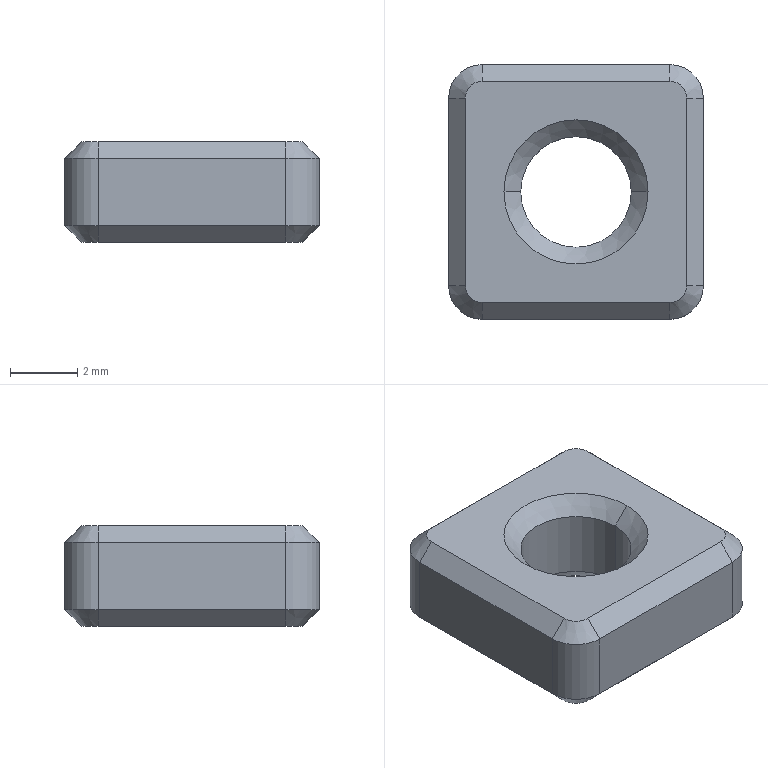Part | SolidWorks | features Chamfer 3, Extrusion 1, HoleWzd 1 | 1 solid | 32 faces | box 7.6 x 7.6 x 3 mm | volume 135.283 mm3 | plane 14 | cone 12 | cylinder 6 | commonest cylinder face diameters 2 x4 3.3 x2
STEP:
#1=CARTESIAN_POINT('',(-1.65,0.,2.5));
#2=VERTEX_POINT('',#1);
#3=CARTESIAN_POINT('',(1.65,0.,2.5));
#4=VERTEX_POINT('',#3);
#5=CARTESIAN_POINT('',(0.,0.,2.5));
#6=DIRECTION('',(0.,0.,1.));
#7=DIRECTION('',(1.,0.,0.));
#8=AXIS2_PLACEMENT_3D('',#5,#6,#7);
#9=CIRCLE('',#8,1.65);
#10=EDGE_CURVE('',#2,#4,#9,.T.);
#11=ORIENTED_EDGE('',*,*,#10,.F.);
#12=CARTESIAN_POINT('',(-2.15,0.,3.));
#13=VERTEX_POINT('',#12);
#14=CARTESIAN_POINT('',(-1.65,0.,2.5));
#15=DIRECTION('',(-0.7071,0.,0.7071));
#16=VECTOR('',#15,1000.);
#17=LINE('',#14,#16);
#18=EDGE_CURVE('',#2,#13,#17,.T.);
#19=ORIENTED_EDGE('',*,*,#18,.T.);
#20=CARTESIAN_POINT('',(2.15,0.,3.));
#21=VERTEX_POINT('',#20);
#22=CARTESIAN_POINT('',(0.,0.,3.));
#23=DIRECTION('',(0.,0.,-1.));
#24=DIRECTION('',(1.,0.,0.));
#25=AXIS2_PLACEMENT_3D('',#22,#23,#24);
#26=CIRCLE('',#25,2.15);
#27=EDGE_CURVE('',#21,#13,#26,.T.);
#28=ORIENTED_EDGE('',*,*,#27,.F.);
#29=CARTESIAN_POINT('',(1.65,0.,2.5));
#30=DIRECTION('',(0.7071,0.,0.7071));
#31=VECTOR('',#30,1000.);
#32=LINE('',#29,#31);
#33=EDGE_CURVE('',#4,#21,#32,.T.);
#34=ORIENTED_EDGE('',*,*,#33,.F.);
#35=EDGE_LOOP('',(#11,#19,#28,#34));
#36=FACE_OUTER_BOUND('',#35,.T.);
#37=CARTESIAN_POINT('',(0.,0.,2.5));
#38=DIRECTION('',(0.,0.,1.));
#39=DIRECTION('',(1.,0.,0.));
#40=AXIS2_PLACEMENT_3D('',#37,#38,#39);
#41=CONICAL_SURFACE('',#40,1.65,0.7854);
#42=ADVANCED_FACE('',(#36),#41,.F.);
#43=CARTESIAN_POINT('',(1.65,0.,0.5));
#44=VERTEX_POINT('',#43);
#45=CARTESIAN_POINT('',(-1.65,0.,0.5));
#46=VERTEX_POINT('',#45);
#47=CARTESIAN_POINT('',(0.,0.,0.5));
#48=DIRECTION('',(0.,0.,-1.));
#49=DIRECTION('',(1.,0.,0.));
#50=AXIS2_PLACEMENT_3D('',#47,#48,#49);
#51=CIRCLE('',#50,1.65);
#52=EDGE_CURVE('',#44,#46,#51,.T.);
#53=ORIENTED_EDGE('',*,*,#52,.F.);
#54=CARTESIAN_POINT('',(2.15,0.,0.));
#55=VERTEX_POINT('',#54);
#56=CARTESIAN_POINT('',(1.65,0.,0.5));
#57=DIRECTION('',(0.7071,0.,-0.7071));
#58=VECTOR('',#57,1000.);
#59=LINE('',#56,#58);
#60=EDGE_CURVE('',#44,#55,#59,.T.);
#61=ORIENTED_EDGE('',*,*,#60,.T.);
#62=CARTESIAN_POINT('',(-2.15,0.,0.));
#63=VERTEX_POINT('',#62);
#64=CARTESIAN_POINT('',(0.,0.,0.));
#65=DIRECTION('',(0.,0.,1.));
#66=DIRECTION('',(1.,0.,0.));
#67=AXIS2_PLACEMENT_3D('',#64,#65,#66);
#68=CIRCLE('',#67,2.15);
#69=EDGE_CURVE('',#63,#55,#68,.T.);
#70=ORIENTED_EDGE('',*,*,#69,.F.);
#71=CARTESIAN_POINT('',(-1.65,0.,0.5));
#72=DIRECTION('',(-0.7071,0.,-0.7071));
#73=VECTOR('',#72,1000.);
#74=LINE('',#71,#73);
#75=EDGE_CURVE('',#46,#63,#74,.T.);
#76=ORIENTED_EDGE('',*,*,#75,.F.);
#77=EDGE_LOOP('',(#53,#61,#70,#76));
#78=FACE_OUTER_BOUND('',#77,.T.);
#79=CARTESIAN_POINT('',(0.,0.,0.5));
#80=DIRECTION('',(0.,0.,-1.));
#81=DIRECTION('',(-1.,0.,0.));
#82=AXIS2_PLACEMENT_3D('',#79,#80,#81);
#83=CONICAL_SURFACE('',#82,1.65,0.7854);
#84=ADVANCED_FACE('',(#78),#83,.F.);
#85=ORIENTED_EDGE('',*,*,#10,.T.);
#86=CARTESIAN_POINT('',(1.65,0.,0.));
#87=DIRECTION('',(0.,0.,-1.));
#88=VECTOR('',#87,1000.);
#89=LINE('',#86,#88);
#90=EDGE_CURVE('',#4,#44,#89,.T.);
#91=ORIENTED_EDGE('',*,*,#90,.T.);
#92=ORIENTED_EDGE('',*,*,#52,.T.);
#93=CARTESIAN_POINT('',(-1.65,0.,0.));
#94=DIRECTION('',(0.,0.,-1.));
#95=VECTOR('',#94,1000.);
#96=LINE('',#93,#95);
#97=EDGE_CURVE('',#2,#46,#96,.T.);
#98=ORIENTED_EDGE('',*,*,#97,.F.);
#99=EDGE_LOOP('',(#85,#91,#92,#98));
#100=FACE_OUTER_BOUND('',#99,.T.);
#101=CARTESIAN_POINT('',(0.,0.,0.));
#102=DIRECTION('',(0.,0.,-1.));
#103=DIRECTION('',(-1.,0.,0.));
#104=AXIS2_PLACEMENT_3D('',#101,#102,#103);
#105=CYLINDRICAL_SURFACE('',#104,1.65);
#106=ADVANCED_FACE('',(#100),#105,.F.);
#107=CARTESIAN_POINT('',(3.3,2.8,0.));
#108=VERTEX_POINT('',#107);
#109=CARTESIAN_POINT('',(3.3,-2.8,0.));
#110=VERTEX_POINT('',#109);
#111=CARTESIAN_POINT('',(3.3,-2.8,0.));
#112=DIRECTION('',(0.,-1.,0.));
#113=VECTOR('',#112,1000.);
#114=LINE('',#111,#113);
#115=EDGE_CURVE('',#108,#110,#114,.T.);
#116=ORIENTED_EDGE('',*,*,#115,.T.);
#117=CARTESIAN_POINT('',(2.8,-3.3,0.));
#118=VERTEX_POINT('',#117);
#119=CARTESIAN_POINT('',(2.8,-2.8,0.));
#120=DIRECTION('',(0.,0.,-1.));
#121=DIRECTION('',(1.,0.,0.));
#122=AXIS2_PLACEMENT_3D('',#119,#120,#121);
#123=CIRCLE('',#122,0.5);
#124=EDGE_CURVE('',#110,#118,#123,.T.);
#125=ORIENTED_EDGE('',*,*,#124,.T.);
#126=CARTESIAN_POINT('',(-2.8,-3.3,0.));
#127=VERTEX_POINT('',#126);
#128=CARTESIAN_POINT('',(-2.8,-3.3,0.));
#129=DIRECTION('',(-1.,0.,0.));
#130=VECTOR('',#129,1000.);
#131=LINE('',#128,#130);
#132=EDGE_CURVE('',#118,#127,#131,.T.);
#133=ORIENTED_EDGE('',*,*,#132,.T.);
#134=CARTESIAN_POINT('',(-3.3,-2.8,0.));
#135=VERTEX_POINT('',#134);
#136=CARTESIAN_POINT('',(-2.8,-2.8,0.));
#137=DIRECTION('',(0.,0.,-1.));
#138=DIRECTION('',(1.,0.,0.));
#139=AXIS2_PLACEMENT_3D('',#136,#137,#138);
#140=CIRCLE('',#139,0.5);
#141=EDGE_CURVE('',#127,#135,#140,.T.);
#142=ORIENTED_EDGE('',*,*,#141,.T.);
#143=CARTESIAN_POINT('',(-3.3,2.8,0.));
#144=VERTEX_POINT('',#143);
#145=CARTESIAN_POINT('',(-3.3,-2.8,0.));
#146=DIRECTION('',(0.,1.,0.));
#147=VECTOR('',#146,1000.);
#148=LINE('',#145,#147);
#149=EDGE_CURVE('',#135,#144,#148,.T.);
#150=ORIENTED_EDGE('',*,*,#149,.T.);
#151=CARTESIAN_POINT('',(-2.8,3.3,0.));
#152=VERTEX_POINT('',#151);
#153=CARTESIAN_POINT('',(-2.8,2.8,0.));
#154=DIRECTION('',(0.,0.,-1.));
#155=DIRECTION('',(1.,0.,0.));
#156=AXIS2_PLACEMENT_3D('',#153,#154,#155);
#157=CIRCLE('',#156,0.5);
#158=EDGE_CURVE('',#144,#152,#157,.T.);
#159=ORIENTED_EDGE('',*,*,#158,.T.);
#160=CARTESIAN_POINT('',(2.8,3.3,0.));
#161=VERTEX_POINT('',#160);
#162=CARTESIAN_POINT('',(-2.8,3.3,0.));
#163=DIRECTION('',(1.,0.,0.));
#164=VECTOR('',#163,1000.);
#165=LINE('',#162,#164);
#166=EDGE_CURVE('',#152,#161,#165,.T.);
#167=ORIENTED_EDGE('',*,*,#166,.T.);
#168=CARTESIAN_POINT('',(2.8,2.8,0.));
#169=DIRECTION('',(0.,0.,-1.));
#170=DIRECTION('',(1.,0.,0.));
#171=AXIS2_PLACEMENT_3D('',#168,#169,#170);
#172=CIRCLE('',#171,0.5);
#173=EDGE_CURVE('',#161,#108,#172,.T.);
#174=ORIENTED_EDGE('',*,*,#173,.T.);
#175=EDGE_LOOP('',(#116,#125,#133,#142,#150,#159,#167,#174));
#176=FACE_OUTER_BOUND('',#175,.T.);
#177=ORIENTED_EDGE('',*,*,#69,.T.);
#178=CARTESIAN_POINT('',(0.,0.,0.));
#179=DIRECTION('',(0.,0.,1.));
#180=DIRECTION('',(1.,0.,0.));
#181=AXIS2_PLACEMENT_3D('',#178,#179,#180);
#182=CIRCLE('',#181,2.15);
#183=EDGE_CURVE('',#55,#63,#182,.T.);
#184=ORIENTED_EDGE('',*,*,#183,.T.);
#185=EDGE_LOOP('',(#177,#184));
#186=FACE_BOUND('',#185,.T.);
#187=CARTESIAN_POINT('',(-2.8,-2.8,0.));
#188=DIRECTION('',(0.,0.,1.));
#189=DIRECTION('',(1.,0.,0.));
#190=AXIS2_PLACEMENT_3D('',#187,#188,#189);
#191=PLANE('',#190);
#192=ADVANCED_FACE('',(#176,#186),#191,.F.);
#193=CARTESIAN_POINT('',(2.8,3.3,3.));
#194=VERTEX_POINT('',#193);
#195=CARTESIAN_POINT('',(-2.8,3.3,3.));
#196=VERTEX_POINT('',#195);
#197=CARTESIAN_POINT('',(-2.8,3.3,3.));
#198=DIRECTION('',(-1.,0.,0.));
#199=VECTOR('',#198,1000.);
#200=LINE('',#197,#199);
#201=EDGE_CURVE('',#194,#196,#200,.T.);
#202=ORIENTED_EDGE('',*,*,#201,.T.);
#203=CARTESIAN_POINT('',(-3.3,2.8,3.));
#204=VERTEX_POINT('',#203);
#205=CARTESIAN_POINT('',(-2.8,2.8,3.));
#206=DIRECTION('',(0.,0.,1.));
#207=DIRECTION('',(1.,0.,0.));
#208=AXIS2_PLACEMENT_3D('',#205,#206,#207);
#209=CIRCLE('',#208,0.5);
#210=EDGE_CURVE('',#196,#204,#209,.T.);
#211=ORIENTED_EDGE('',*,*,#210,.T.);
#212=CARTESIAN_POINT('',(-3.3,-2.8,3.));
#213=VERTEX_POINT('',#212);
#214=CARTESIAN_POINT('',(-3.3,-2.8,3.));
#215=DIRECTION('',(0.,-1.,0.));
#216=VECTOR('',#215,1000.);
#217=LINE('',#214,#216);
#218=EDGE_CURVE('',#204,#213,#217,.T.);
#219=ORIENTED_EDGE('',*,*,#218,.T.);
#220=CARTESIAN_POINT('',(-2.8,-3.3,3.));
#221=VERTEX_POINT('',#220);
#222=CARTESIAN_POINT('',(-2.8,-2.8,3.));
#223=DIRECTION('',(0.,0.,1.));
#224=DIRECTION('',(1.,0.,0.));
#225=AXIS2_PLACEMENT_3D('',#222,#223,#224);
#226=CIRCLE('',#225,0.5);
#227=EDGE_CURVE('',#213,#221,#226,.T.);
#228=ORIENTED_EDGE('',*,*,#227,.T.);
#229=CARTESIAN_POINT('',(2.8,-3.3,3.));
#230=VERTEX_POINT('',#229);
#231=CARTESIAN_POINT('',(2.8,-3.3,3.));
#232=DIRECTION('',(1.,0.,0.));
#233=VECTOR('',#232,1000.);
#234=LINE('',#231,#233);
#235=EDGE_CURVE('',#221,#230,#234,.T.);
#236=ORIENTED_EDGE('',*,*,#235,.T.);
#237=CARTESIAN_POINT('',(3.3,-2.8,3.));
#238=VERTEX_POINT('',#237);
#239=CARTESIAN_POINT('',(2.8,-2.8,3.));
#240=DIRECTION('',(0.,0.,1.));
#241=DIRECTION('',(1.,0.,0.));
#242=AXIS2_PLACEMENT_3D('',#239,#240,#241);
#243=CIRCLE('',#242,0.5);
#244=EDGE_CURVE('',#230,#238,#243,.T.);
#245=ORIENTED_EDGE('',*,*,#244,.T.);
#246=CARTESIAN_POINT('',(3.3,2.8,3.));
#247=VERTEX_POINT('',#246);
#248=CARTESIAN_POINT('',(3.3,2.8,3.));
#249=DIRECTION('',(0.,1.,0.));
#250=VECTOR('',#249,1000.);
#251=LINE('',#248,#250);
#252=EDGE_CURVE('',#238,#247,#251,.T.);
#253=ORIENTED_EDGE('',*,*,#252,.T.);
#254=CARTESIAN_POINT('',(2.8,2.8,3.));
#255=DIRECTION('',(0.,0.,1.));
#256=DIRECTION('',(1.,0.,0.));
#257=AXIS2_PLACEMENT_3D('',#254,#255,#256);
#258=CIRCLE('',#257,0.5);
#259=EDGE_CURVE('',#247,#194,#258,.T.);
#260=ORIENTED_EDGE('',*,*,#259,.T.);
#261=EDGE_LOOP('',(#202,#211,#219,#228,#236,#245,#253,#260));
#262=FACE_OUTER_BOUND('',#261,.T.);
#263=ORIENTED_EDGE('',*,*,#27,.T.);
#264=CARTESIAN_POINT('',(0.,0.,3.));
#265=DIRECTION('',(0.,0.,-1.));
#266=DIRECTION('',(1.,0.,0.));
#267=AXIS2_PLACEMENT_3D('',#264,#265,#266);
#268=CIRCLE('',#267,2.15);
#269=EDGE_CURVE('',#13,#21,#268,.T.);
#270=ORIENTED_EDGE('',*,*,#269,.T.);
#271=EDGE_LOOP('',(#263,#270));
#272=FACE_BOUND('',#271,.T.);
#273=CARTESIAN_POINT('',(-2.8,-2.8,3.));
#274=DIRECTION('',(0.,0.,1.));
#275=DIRECTION('',(1.,0.,0.));
#276=AXIS2_PLACEMENT_3D('',#273,#274,#275);
#277=PLANE('',#276);
#278=ADVANCED_FACE('',(#262,#272),#277,.T.);
#279=CARTESIAN_POINT('',(-2.8,-3.8,2.5));
#280=VERTEX_POINT('',#279);
#281=CARTESIAN_POINT('',(-2.8,-3.8,0.5));
#282=VERTEX_POINT('',#281);
#283=CARTESIAN_POINT('',(-2.8,-3.8,3.));
#284=DIRECTION('',(0.,0.,-1.));
#285=VECTOR('',#284,1000.);
#286=LINE('',#283,#285);
#287=EDGE_CURVE('',#280,#282,#286,.T.);
#288=ORIENTED_EDGE('',*,*,#287,.F.);
#289=CARTESIAN_POINT('',(-3.8,-2.8,2.5));
#290=VERTEX_POINT('',#289);
#291=CARTESIAN_POINT('',(-2.8,-2.8,2.5));
#292=DIRECTION('',(0.,0.,-1.));
#293=DIRECTION('',(1.,0.,0.));
#294=AXIS2_PLACEMENT_3D('',#291,#292,#293);
#295=CIRCLE('',#294,1.);
#296=EDGE_CURVE('',#280,#290,#295,.T.);
#297=ORIENTED_EDGE('',*,*,#296,.T.);
#298=CARTESIAN_POINT('',(-3.8,-2.8,0.5));
#299=VERTEX_POINT('',#298);
#300=CARTESIAN_POINT('',(-3.8,-2.8,3.));
#301=DIRECTION('',(0.,0.,-1.));
#302=VECTOR('',#301,1000.);
#303=LINE('',#300,#302);
#304=EDGE_CURVE('',#290,#299,#303,.T.);
#305=ORIENTED_EDGE('',*,*,#304,.T.);
#306=CARTESIAN_POINT('',(-2.8,-2.8,0.5));
#307=DIRECTION('',(0.,0.,1.));
#308=DIRECTION('',(1.,0.,0.));
#309=AXIS2_PLACEMENT_3D('',#306,#307,#308);
#310=CIRCLE('',#309,1.);
#311=EDGE_CURVE('',#299,#282,#310,.T.);
#312=ORIENTED_EDGE('',*,*,#311,.T.);
#313=EDGE_LOOP('',(#288,#297,#305,#312));
#314=FACE_OUTER_BOUND('',#313,.T.);
#315=CARTESIAN_POINT('',(-2.8,-2.8,3.));
#316=DIRECTION('',(0.,0.,-1.));
#317=DIRECTION('',(-1.,0.,0.));
#318=AXIS2_PLACEMENT_3D('',#315,#316,#317);
#319=CYLINDRICAL_SURFACE('',#318,1.);
#320=ADVANCED_FACE('',(#314),#319,.T.);
#321=CARTESIAN_POINT('',(2.8,-3.8,2.5));
#322=VERTEX_POINT('',#321);
#323=CARTESIAN_POINT('',(2.8,-3.8,0.5));
#324=VERTEX_POINT('',#323);
#325=CARTESIAN_POINT('',(2.8,-3.8,3.));
#326=DIRECTION('',(0.,0.,-1.));
#327=VECTOR('',#326,1000.);
#328=LINE('',#325,#327);
#329=EDGE_CURVE('',#322,#324,#328,.T.);
#330=ORIENTED_EDGE('',*,*,#329,.F.);
#331=CARTESIAN_POINT('',(-2.8,-3.8,2.5));
#332=DIRECTION('',(-1.,0.,0.));
#333=VECTOR('',#332,1000.);
#334=LINE('',#331,#333);
#335=EDGE_CURVE('',#322,#280,#334,.T.);
#336=ORIENTED_EDGE('',*,*,#335,.T.);
#337=ORIENTED_EDGE('',*,*,#287,.T.);
#338=CARTESIAN_POINT('',(-2.8,-3.8,0.5));
#339=DIRECTION('',(1.,0.,0.));
#340=VECTOR('',#339,1000.);
#341=LINE('',#338,#340);
#342=EDGE_CURVE('',#282,#324,#341,.T.);
#343=ORIENTED_EDGE('',*,*,#342,.T.);
#344=EDGE_LOOP('',(#330,#336,#337,#343));
#345=FACE_OUTER_BOUND('',#344,.T.);
#346=CARTESIAN_POINT('',(-2.8,-3.8,3.));
#347=DIRECTION('',(0.,1.,0.));
#348=DIRECTION('',(0.,0.,1.));
#349=AXIS2_PLACEMENT_3D('',#346,#347,#348);
#350=PLANE('',#349);
#351=ADVANCED_FACE('',(#345),#350,.F.);
#352=CARTESIAN_POINT('',(3.8,-2.8,2.5));
#353=VERTEX_POINT('',#352);
#354=CARTESIAN_POINT('',(3.8,-2.8,0.5));
#355=VERTEX_POINT('',#354);
#356=CARTESIAN_POINT('',(3.8,-2.8,3.));
#357=DIRECTION('',(0.,0.,-1.));
#358=VECTOR('',#357,1000.);
#359=LINE('',#356,#358);
#360=EDGE_CURVE('',#353,#355,#359,.T.);
#361=ORIENTED_EDGE('',*,*,#360,.F.);
#362=CARTESIAN_POINT('',(2.8,-2.8,2.5));
#363=DIRECTION('',(0.,0.,-1.));
#364=DIRECTION('',(1.,0.,0.));
#365=AXIS2_PLACEMENT_3D('',#362,#363,#364);
#366=CIRCLE('',#365,1.);
#367=EDGE_CURVE('',#353,#322,#366,.T.);
#368=ORIENTED_EDGE('',*,*,#367,.T.);
#369=ORIENTED_EDGE('',*,*,#329,.T.);
#370=CARTESIAN_POINT('',(2.8,-2.8,0.5));
#371=DIRECTION('',(0.,0.,1.));
#372=DIRECTION('',(1.,0.,0.));
#373=AXIS2_PLACEMENT_3D('',#370,#371,#372);
#374=CIRCLE('',#373,1.);
#375=EDGE_CURVE('',#324,#355,#374,.T.);
#376=ORIENTED_EDGE('',*,*,#375,.T.);
#377=EDGE_LOOP('',(#361,#368,#369,#376));
#378=FACE_OUTER_BOUND('',#377,.T.);
#379=CARTESIAN_POINT('',(2.8,-2.8,3.));
#380=DIRECTION('',(0.,0.,-1.));
#381=DIRECTION('',(-1.,0.,0.));
#382=AXIS2_PLACEMENT_3D('',#379,#380,#381);
#383=CYLINDRICAL_SURFACE('',#382,1.);
#384=ADVANCED_FACE('',(#378),#383,.T.);
#385=CARTESIAN_POINT('',(3.8,2.8,2.5));
#386=VERTEX_POINT('',#385);
#387=CARTESIAN_POINT('',(3.8,2.8,0.5));
#388=VERTEX_POINT('',#387);
#389=CARTESIAN_POINT('',(3.8,2.8,3.));
#390=DIRECTION('',(0.,0.,-1.));
#391=VECTOR('',#390,1000.);
#392=LINE('',#389,#391);
#393=EDGE_CURVE('',#386,#388,#392,.T.);
#394=ORIENTED_EDGE('',*,*,#393,.F.);
#395=CARTESIAN_POINT('',(3.8,-2.8,2.5));
#396=DIRECTION('',(0.,-1.,0.));
#397=VECTOR('',#396,1000.);
#398=LINE('',#395,#397);
#399=EDGE_CURVE('',#386,#353,#398,.T.);
#400=ORIENTED_EDGE('',*,*,#399,.T.);
#401=ORIENTED_EDGE('',*,*,#360,.T.);
#402=CARTESIAN_POINT('',(3.8,2.8,0.5));
#403=DIRECTION('',(0.,1.,0.));
#404=VECTOR('',#403,1000.);
#405=LINE('',#402,#404);
#406=EDGE_CURVE('',#355,#388,#405,.T.);
#407=ORIENTED_EDGE('',*,*,#406,.T.);
#408=EDGE_LOOP('',(#394,#400,#401,#407));
#409=FACE_OUTER_BOUND('',#408,.T.);
#410=CARTESIAN_POINT('',(3.8,2.8,3.));
#411=DIRECTION('',(-1.,0.,0.));
#412=DIRECTION('',(0.,-1.,0.));
#413=AXIS2_PLACEMENT_3D('',#410,#411,#412);
#414=PLANE('',#413);
#415=ADVANCED_FACE('',(#409),#414,.F.);
#416=CARTESIAN_POINT('',(2.8,3.8,2.5));
#417=VERTEX_POINT('',#416);
#418=CARTESIAN_POINT('',(2.8,3.8,0.5));
#419=VERTEX_POINT('',#418);
#420=CARTESIAN_POINT('',(2.8,3.8,3.));
#421=DIRECTION('',(0.,0.,-1.));
#422=VECTOR('',#421,1000.);
#423=LINE('',#420,#422);
#424=EDGE_CURVE('',#417,#419,#423,.T.);
#425=ORIENTED_EDGE('',*,*,#424,.F.);
#426=CARTESIAN_POINT('',(2.8,2.8,2.5));
#427=DIRECTION('',(0.,0.,-1.));
#428=DIRECTION('',(1.,0.,0.));
#429=AXIS2_PLACEMENT_3D('',#426,#427,#428);
#430=CIRCLE('',#429,1.);
#431=EDGE_CURVE('',#417,#386,#430,.T.);
#432=ORIENTED_EDGE('',*,*,#431,.T.);
#433=ORIENTED_EDGE('',*,*,#393,.T.);
#434=CARTESIAN_POINT('',(2.8,2.8,0.5));
#435=DIRECTION('',(0.,0.,1.));
#436=DIRECTION('',(1.,0.,0.));
#437=AXIS2_PLACEMENT_3D('',#434,#435,#436);
#438=CIRCLE('',#437,1.);
#439=EDGE_CURVE('',#388,#419,#438,.T.);
#440=ORIENTED_EDGE('',*,*,#439,.T.);
#441=EDGE_LOOP('',(#425,#432,#433,#440));
#442=FACE_OUTER_BOUND('',#441,.T.);
#443=CARTESIAN_POINT('',(2.8,2.8,3.));
#444=DIRECTION('',(0.,0.,-1.));
#445=DIRECTION('',(-1.,0.,0.));
#446=AXIS2_PLACEMENT_3D('',#443,#444,#445);
#447=CYLINDRICAL_SURFACE('',#446,1.);
#448=ADVANCED_FACE('',(#442),#447,.T.);
#449=CARTESIAN_POINT('',(-2.8,3.8,2.5));
#450=VERTEX_POINT('',#449);
#451=CARTESIAN_POINT('',(-2.8,3.8,0.5));
#452=VERTEX_POINT('',#451);
#453=CARTESIAN_POINT('',(-2.8,3.8,3.));
#454=DIRECTION('',(0.,0.,-1.));
#455=VECTOR('',#454,1000.);
#456=LINE('',#453,#455);
#457=EDGE_CURVE('',#450,#452,#456,.T.);
#458=ORIENTED_EDGE('',*,*,#457,.F.);
#459=CARTESIAN_POINT('',(2.8,3.8,2.5));
#460=DIRECTION('',(1.,0.,0.));
#461=VECTOR('',#460,1000.);
#462=LINE('',#459,#461);
#463=EDGE_CURVE('',#450,#417,#462,.T.);
#464=ORIENTED_EDGE('',*,*,#463,.T.);
#465=ORIENTED_EDGE('',*,*,#424,.T.);
#466=CARTESIAN_POINT('',(-2.8,3.8,0.5));
#467=DIRECTION('',(-1.,0.,0.));
#468=VECTOR('',#467,1000.);
#469=LINE('',#466,#468);
#470=EDGE_CURVE('',#419,#452,#469,.T.);
#471=ORIENTED_EDGE('',*,*,#470,.T.);
#472=EDGE_LOOP('',(#458,#464,#465,#471));
#473=FACE_OUTER_BOUND('',#472,.T.);
#474=CARTESIAN_POINT('',(-2.8,3.8,3.));
#475=DIRECTION('',(0.,-1.,0.));
#476=DIRECTION('',(0.,0.,-1.));
#477=AXIS2_PLACEMENT_3D('',#474,#475,#476);
#478=PLANE('',#477);
#479=ADVANCED_FACE('',(#473),#478,.F.);
#480=CARTESIAN_POINT('',(-3.8,2.8,2.5));
#481=VERTEX_POINT('',#480);
#482=CARTESIAN_POINT('',(-3.8,2.8,0.5));
#483=VERTEX_POINT('',#482);
#484=CARTESIAN_POINT('',(-3.8,2.8,3.));
#485=DIRECTION('',(0.,0.,-1.));
#486=VECTOR('',#485,1000.);
#487=LINE('',#484,#486);
#488=EDGE_CURVE('',#481,#483,#487,.T.);
#489=ORIENTED_EDGE('',*,*,#488,.F.);
#490=CARTESIAN_POINT('',(-2.8,2.8,2.5));
#491=DIRECTION('',(0.,0.,-1.));
#492=DIRECTION('',(1.,0.,0.));
#493=AXIS2_PLACEMENT_3D('',#490,#491,#492);
#494=CIRCLE('',#493,1.);
#495=EDGE_CURVE('',#481,#450,#494,.T.);
#496=ORIENTED_EDGE('',*,*,#495,.T.);
#497=ORIENTED_EDGE('',*,*,#457,.T.);
#498=CARTESIAN_POINT('',(-2.8,2.8,0.5));
#499=DIRECTION('',(0.,0.,1.));
#500=DIRECTION('',(1.,0.,0.));
#501=AXIS2_PLACEMENT_3D('',#498,#499,#500);
#502=CIRCLE('',#501,1.);
#503=EDGE_CURVE('',#452,#483,#502,.T.);
#504=ORIENTED_EDGE('',*,*,#503,.T.);
#505=EDGE_LOOP('',(#489,#496,#497,#504));
#506=FACE_OUTER_BOUND('',#505,.T.);
#507=CARTESIAN_POINT('',(-2.8,2.8,3.));
#508=DIRECTION('',(0.,0.,-1.));
#509=DIRECTION('',(-1.,0.,0.));
#510=AXIS2_PLACEMENT_3D('',#507,#508,#509);
#511=CYLINDRICAL_SURFACE('',#510,1.);
#512=ADVANCED_FACE('',(#506),#511,.T.);
#513=ORIENTED_EDGE('',*,*,#304,.F.);
#514=CARTESIAN_POINT('',(-3.8,2.8,2.5));
#515=DIRECTION('',(0.,1.,0.));
#516=VECTOR('',#515,1000.);
#517=LINE('',#514,#516);
#518=EDGE_CURVE('',#290,#481,#517,.T.);
#519=ORIENTED_EDGE('',*,*,#518,.T.);
#520=ORIENTED_EDGE('',*,*,#488,.T.);
#521=CARTESIAN_POINT('',(-3.8,2.8,0.5));
#522=DIRECTION('',(0.,-1.,0.));
#523=VECTOR('',#522,1000.);
#524=LINE('',#521,#523);
#525=EDGE_CURVE('',#483,#299,#524,.T.);
#526=ORIENTED_EDGE('',*,*,#525,.T.);
#527=EDGE_LOOP('',(#513,#519,#520,#526));
#528=FACE_OUTER_BOUND('',#527,.T.);
#529=CARTESIAN_POINT('',(-3.8,2.8,3.));
#530=DIRECTION('',(1.,0.,0.));
#531=DIRECTION('',(0.,1.,0.));
#532=AXIS2_PLACEMENT_3D('',#529,#530,#531);
#533=PLANE('',#532);
#534=ADVANCED_FACE('',(#528),#533,.F.);
#535=ORIENTED_EDGE('',*,*,#90,.F.);
#536=CARTESIAN_POINT('',(0.,0.,2.5));
#537=DIRECTION('',(0.,0.,1.));
#538=DIRECTION('',(1.,0.,0.));
#539=AXIS2_PLACEMENT_3D('',#536,#537,#538);
#540=CIRCLE('',#539,1.65);
#541=EDGE_CURVE('',#4,#2,#540,.T.);
#542=ORIENTED_EDGE('',*,*,#541,.T.);
#543=ORIENTED_EDGE('',*,*,#97,.T.);
#544=CARTESIAN_POINT('',(0.,0.,0.5));
#545=DIRECTION('',(0.,0.,-1.));
#546=DIRECTION('',(1.,0.,0.));
#547=AXIS2_PLACEMENT_3D('',#544,#545,#546);
#548=CIRCLE('',#547,1.65);
#549=EDGE_CURVE('',#46,#44,#548,.T.);
#550=ORIENTED_EDGE('',*,*,#549,.T.);
#551=EDGE_LOOP('',(#535,#542,#543,#550));
#552=FACE_OUTER_BOUND('',#551,.T.);
#553=CARTESIAN_POINT('',(0.,0.,0.));
#554=DIRECTION('',(0.,0.,-1.));
#555=DIRECTION('',(-1.,0.,0.));
#556=AXIS2_PLACEMENT_3D('',#553,#554,#555);
#557=CYLINDRICAL_SURFACE('',#556,1.65);
#558=ADVANCED_FACE('',(#552),#557,.F.);
#559=ORIENTED_EDGE('',*,*,#60,.F.);
#560=ORIENTED_EDGE('',*,*,#549,.F.);
#561=ORIENTED_EDGE('',*,*,#75,.T.);
#562=ORIENTED_EDGE('',*,*,#183,.F.);
#563=EDGE_LOOP('',(#559,#560,#561,#562));
#564=FACE_OUTER_BOUND('',#563,.T.);
#565=CARTESIAN_POINT('',(0.,0.,0.5));
#566=DIRECTION('',(0.,0.,-1.));
#567=DIRECTION('',(-1.,0.,0.));
#568=AXIS2_PLACEMENT_3D('',#565,#566,#567);
#569=CONICAL_SURFACE('',#568,1.65,0.7854);
#570=ADVANCED_FACE('',(#564),#569,.F.);
#571=ORIENTED_EDGE('',*,*,#18,.F.);
#572=ORIENTED_EDGE('',*,*,#541,.F.);
#573=ORIENTED_EDGE('',*,*,#33,.T.);
#574=ORIENTED_EDGE('',*,*,#269,.F.);
#575=EDGE_LOOP('',(#571,#572,#573,#574));
#576=FACE_OUTER_BOUND('',#575,.T.);
#577=CARTESIAN_POINT('',(0.,0.,2.5));
#578=DIRECTION('',(0.,0.,1.));
#579=DIRECTION('',(1.,0.,0.));
#580=AXIS2_PLACEMENT_3D('',#577,#578,#579);
#581=CONICAL_SURFACE('',#580,1.65,0.7854);
#582=ADVANCED_FACE('',(#576),#581,.F.);
#583=CARTESIAN_POINT('',(2.8,-3.8,2.5));
#584=DIRECTION('',(0.,0.7071,0.7071));
#585=VECTOR('',#584,1000.);
#586=LINE('',#583,#585);
#587=EDGE_CURVE('',#322,#230,#586,.T.);
#588=ORIENTED_EDGE('',*,*,#587,.F.);
#589=ORIENTED_EDGE('',*,*,#367,.F.);
#590=CARTESIAN_POINT('',(3.3,-2.8,3.));
#591=DIRECTION('',(0.7071,0.,-0.7071));
#592=VECTOR('',#591,1000.);
#593=LINE('',#590,#592);
#594=EDGE_CURVE('',#238,#353,#593,.T.);
#595=ORIENTED_EDGE('',*,*,#594,.F.);
#596=ORIENTED_EDGE('',*,*,#244,.F.);
#597=EDGE_LOOP('',(#588,#589,#595,#596));
#598=FACE_OUTER_BOUND('',#597,.T.);
#599=CARTESIAN_POINT('',(2.8,-2.8,3.));
#600=DIRECTION('',(0.,0.,-1.));
#601=DIRECTION('',(-1.,0.,0.));
#602=AXIS2_PLACEMENT_3D('',#599,#600,#601);
#603=CONICAL_SURFACE('',#602,0.5,0.7854);
#604=ADVANCED_FACE('',(#598),#603,.T.);
#605=ORIENTED_EDGE('',*,*,#594,.T.);
#606=ORIENTED_EDGE('',*,*,#399,.F.);
#607=CARTESIAN_POINT('',(3.3,2.8,3.));
#608=DIRECTION('',(0.7071,0.,-0.7071));
#609=VECTOR('',#608,1000.);
#610=LINE('',#607,#609);
#611=EDGE_CURVE('',#247,#386,#610,.T.);
#612=ORIENTED_EDGE('',*,*,#611,.F.);
#613=ORIENTED_EDGE('',*,*,#252,.F.);
#614=EDGE_LOOP('',(#605,#606,#612,#613));
#615=FACE_OUTER_BOUND('',#614,.T.);
#616=CARTESIAN_POINT('',(3.3,-2.8,3.));
#617=DIRECTION('',(0.7071,0.,0.7071));
#618=DIRECTION('',(0.,-1.,0.));
#619=AXIS2_PLACEMENT_3D('',#616,#617,#618);
#620=PLANE('',#619);
#621=ADVANCED_FACE('',(#615),#620,.T.);
#622=ORIENTED_EDGE('',*,*,#587,.T.);
#623=ORIENTED_EDGE('',*,*,#235,.F.);
#624=CARTESIAN_POINT('',(-2.8,-3.8,2.5));
#625=DIRECTION('',(0.,0.7071,0.7071));
#626=VECTOR('',#625,1000.);
#627=LINE('',#624,#626);
#628=EDGE_CURVE('',#280,#221,#627,.T.);
#629=ORIENTED_EDGE('',*,*,#628,.F.);
#630=ORIENTED_EDGE('',*,*,#335,.F.);
#631=EDGE_LOOP('',(#622,#623,#629,#630));
#632=FACE_OUTER_BOUND('',#631,.T.);
#633=CARTESIAN_POINT('',(-2.8,-3.3,3.));
#634=DIRECTION('',(0.,-0.7071,0.7071));
#635=DIRECTION('',(-1.,0.,0.));
#636=AXIS2_PLACEMENT_3D('',#633,#634,#635);
#637=PLANE('',#636);
#638=ADVANCED_FACE('',(#632),#637,.T.);
#639=ORIENTED_EDGE('',*,*,#611,.T.);
#640=ORIENTED_EDGE('',*,*,#431,.F.);
#641=CARTESIAN_POINT('',(2.8,3.3,3.));
#642=DIRECTION('',(0.,0.7071,-0.7071));
#643=VECTOR('',#642,1000.);
#644=LINE('',#641,#643);
#645=EDGE_CURVE('',#194,#417,#644,.T.);
#646=ORIENTED_EDGE('',*,*,#645,.F.);
#647=ORIENTED_EDGE('',*,*,#259,.F.);
#648=EDGE_LOOP('',(#639,#640,#646,#647));
#649=FACE_OUTER_BOUND('',#648,.T.);
#650=CARTESIAN_POINT('',(2.8,2.8,3.));
#651=DIRECTION('',(0.,0.,-1.));
#652=DIRECTION('',(-1.,0.,0.));
#653=AXIS2_PLACEMENT_3D('',#650,#651,#652);
#654=CONICAL_SURFACE('',#653,0.5,0.7854);
#655=ADVANCED_FACE('',(#649),#654,.T.);
#656=ORIENTED_EDGE('',*,*,#628,.T.);
#657=ORIENTED_EDGE('',*,*,#227,.F.);
#658=CARTESIAN_POINT('',(-3.8,-2.8,2.5));
#659=DIRECTION('',(0.7071,0.,0.7071));
#660=VECTOR('',#659,1000.);
#661=LINE('',#658,#660);
#662=EDGE_CURVE('',#290,#213,#661,.T.);
#663=ORIENTED_EDGE('',*,*,#662,.F.);
#664=ORIENTED_EDGE('',*,*,#296,.F.);
#665=EDGE_LOOP('',(#656,#657,#663,#664));
#666=FACE_OUTER_BOUND('',#665,.T.);
#667=CARTESIAN_POINT('',(-2.8,-2.8,3.));
#668=DIRECTION('',(0.,0.,-1.));
#669=DIRECTION('',(-1.,0.,0.));
#670=AXIS2_PLACEMENT_3D('',#667,#668,#669);
#671=CONICAL_SURFACE('',#670,0.5,0.7854);
#672=ADVANCED_FACE('',(#666),#671,.T.);
#673=ORIENTED_EDGE('',*,*,#645,.T.);
#674=ORIENTED_EDGE('',*,*,#463,.F.);
#675=CARTESIAN_POINT('',(-2.8,3.3,3.));
#676=DIRECTION('',(0.,0.7071,-0.7071));
#677=VECTOR('',#676,1000.);
#678=LINE('',#675,#677);
#679=EDGE_CURVE('',#196,#450,#678,.T.);
#680=ORIENTED_EDGE('',*,*,#679,.F.);
#681=ORIENTED_EDGE('',*,*,#201,.F.);
#682=EDGE_LOOP('',(#673,#674,#680,#681));
#683=FACE_OUTER_BOUND('',#682,.T.);
#684=CARTESIAN_POINT('',(-2.8,3.3,3.));
#685=DIRECTION('',(0.,0.7071,0.7071));
#686=DIRECTION('',(1.,0.,0.));
#687=AXIS2_PLACEMENT_3D('',#684,#685,#686);
#688=PLANE('',#687);
#689=ADVANCED_FACE('',(#683),#688,.T.);
#690=ORIENTED_EDGE('',*,*,#662,.T.);
#691=ORIENTED_EDGE('',*,*,#218,.F.);
#692=CARTESIAN_POINT('',(-3.8,2.8,2.5));
#693=DIRECTION('',(0.7071,0.,0.7071));
#694=VECTOR('',#693,1000.);
#695=LINE('',#692,#694);
#696=EDGE_CURVE('',#481,#204,#695,.T.);
#697=ORIENTED_EDGE('',*,*,#696,.F.);
#698=ORIENTED_EDGE('',*,*,#518,.F.);
#699=EDGE_LOOP('',(#690,#691,#697,#698));
#700=FACE_OUTER_BOUND('',#699,.T.);
#701=CARTESIAN_POINT('',(-3.3,-2.8,3.));
#702=DIRECTION('',(-0.7071,0.,0.7071));
#703=DIRECTION('',(0.,1.,0.));
#704=AXIS2_PLACEMENT_3D('',#701,#702,#703);
#705=PLANE('',#704);
#706=ADVANCED_FACE('',(#700),#705,.T.);
#707=ORIENTED_EDGE('',*,*,#679,.T.);
#708=ORIENTED_EDGE('',*,*,#495,.F.);
#709=ORIENTED_EDGE('',*,*,#696,.T.);
#710=ORIENTED_EDGE('',*,*,#210,.F.);
#711=EDGE_LOOP('',(#707,#708,#709,#710));
#712=FACE_OUTER_BOUND('',#711,.T.);
#713=CARTESIAN_POINT('',(-2.8,2.8,3.));
#714=DIRECTION('',(0.,0.,-1.));
#715=DIRECTION('',(-1.,0.,0.));
#716=AXIS2_PLACEMENT_3D('',#713,#714,#715);
#717=CONICAL_SURFACE('',#716,0.5,0.7854);
#718=ADVANCED_FACE('',(#712),#717,.T.);
#719=CARTESIAN_POINT('',(-2.8,3.3,0.));
#720=DIRECTION('',(0.,0.7071,0.7071));
#721=VECTOR('',#720,1000.);
#722=LINE('',#719,#721);
#723=EDGE_CURVE('',#152,#452,#722,.T.);
#724=ORIENTED_EDGE('',*,*,#723,.F.);
#725=ORIENTED_EDGE('',*,*,#158,.F.);
#726=CARTESIAN_POINT('',(-3.8,2.8,0.5));
#727=DIRECTION('',(0.7071,0.,-0.7071));
#728=VECTOR('',#727,1000.);
#729=LINE('',#726,#728);
#730=EDGE_CURVE('',#483,#144,#729,.T.);
#731=ORIENTED_EDGE('',*,*,#730,.F.);
#732=ORIENTED_EDGE('',*,*,#503,.F.);
#733=EDGE_LOOP('',(#724,#725,#731,#732));
#734=FACE_OUTER_BOUND('',#733,.T.);
#735=CARTESIAN_POINT('',(-2.8,2.8,0.5));
#736=DIRECTION('',(0.,0.,1.));
#737=DIRECTION('',(1.,0.,0.));
#738=AXIS2_PLACEMENT_3D('',#735,#736,#737);
#739=CONICAL_SURFACE('',#738,1.,0.7854);
#740=ADVANCED_FACE('',(#734),#739,.T.);
#741=ORIENTED_EDGE('',*,*,#730,.T.);
#742=ORIENTED_EDGE('',*,*,#149,.F.);
#743=CARTESIAN_POINT('',(-3.8,-2.8,0.5));
#744=DIRECTION('',(0.7071,0.,-0.7071));
#745=VECTOR('',#744,1000.);
#746=LINE('',#743,#745);
#747=EDGE_CURVE('',#299,#135,#746,.T.);
#748=ORIENTED_EDGE('',*,*,#747,.F.);
#749=ORIENTED_EDGE('',*,*,#525,.F.);
#750=EDGE_LOOP('',(#741,#742,#748,#749));
#751=FACE_OUTER_BOUND('',#750,.T.);
#752=CARTESIAN_POINT('',(-3.8,2.8,0.5));
#753=DIRECTION('',(0.7071,0.,0.7071));
#754=DIRECTION('',(0.,-1.,0.));
#755=AXIS2_PLACEMENT_3D('',#752,#753,#754);
#756=PLANE('',#755);
#757=ADVANCED_FACE('',(#751),#756,.F.);
#758=ORIENTED_EDGE('',*,*,#723,.T.);
#759=ORIENTED_EDGE('',*,*,#470,.F.);
#760=CARTESIAN_POINT('',(2.8,3.3,0.));
#761=DIRECTION('',(0.,0.7071,0.7071));
#762=VECTOR('',#761,1000.);
#763=LINE('',#760,#762);
#764=EDGE_CURVE('',#161,#419,#763,.T.);
#765=ORIENTED_EDGE('',*,*,#764,.F.);
#766=ORIENTED_EDGE('',*,*,#166,.F.);
#767=EDGE_LOOP('',(#758,#759,#765,#766));
#768=FACE_OUTER_BOUND('',#767,.T.);
#769=CARTESIAN_POINT('',(-2.8,3.8,0.5));
#770=DIRECTION('',(0.,-0.7071,0.7071));
#771=DIRECTION('',(-1.,0.,0.));
#772=AXIS2_PLACEMENT_3D('',#769,#770,#771);
#773=PLANE('',#772);
#774=ADVANCED_FACE('',(#768),#773,.F.);
#775=ORIENTED_EDGE('',*,*,#747,.T.);
#776=ORIENTED_EDGE('',*,*,#141,.F.);
#777=CARTESIAN_POINT('',(-2.8,-3.8,0.5));
#778=DIRECTION('',(0.,0.7071,-0.7071));
#779=VECTOR('',#778,1000.);
#780=LINE('',#777,#779);
#781=EDGE_CURVE('',#282,#127,#780,.T.);
#782=ORIENTED_EDGE('',*,*,#781,.F.);
#783=ORIENTED_EDGE('',*,*,#311,.F.);
#784=EDGE_LOOP('',(#775,#776,#782,#783));
#785=FACE_OUTER_BOUND('',#784,.T.);
#786=CARTESIAN_POINT('',(-2.8,-2.8,0.5));
#787=DIRECTION('',(0.,0.,1.));
#788=DIRECTION('',(1.,0.,0.));
#789=AXIS2_PLACEMENT_3D('',#786,#787,#788);
#790=CONICAL_SURFACE('',#789,1.,0.7854);
#791=ADVANCED_FACE('',(#785),#790,.T.);
#792=ORIENTED_EDGE('',*,*,#764,.T.);
#793=ORIENTED_EDGE('',*,*,#439,.F.);
#794=CARTESIAN_POINT('',(3.3,2.8,0.));
#795=DIRECTION('',(0.7071,0.,0.7071));
#796=VECTOR('',#795,1000.);
#797=LINE('',#794,#796);
#798=EDGE_CURVE('',#108,#388,#797,.T.);
#799=ORIENTED_EDGE('',*,*,#798,.F.);
#800=ORIENTED_EDGE('',*,*,#173,.F.);
#801=EDGE_LOOP('',(#792,#793,#799,#800));
#802=FACE_OUTER_BOUND('',#801,.T.);
#803=CARTESIAN_POINT('',(2.8,2.8,0.5));
#804=DIRECTION('',(0.,0.,1.));
#805=DIRECTION('',(1.,0.,0.));
#806=AXIS2_PLACEMENT_3D('',#803,#804,#805);
#807=CONICAL_SURFACE('',#806,1.,0.7854);
#808=ADVANCED_FACE('',(#802),#807,.T.);
#809=ORIENTED_EDGE('',*,*,#781,.T.);
#810=ORIENTED_EDGE('',*,*,#132,.F.);
#811=CARTESIAN_POINT('',(2.8,-3.8,0.5));
#812=DIRECTION('',(0.,0.7071,-0.7071));
#813=VECTOR('',#812,1000.);
#814=LINE('',#811,#813);
#815=EDGE_CURVE('',#324,#118,#814,.T.);
#816=ORIENTED_EDGE('',*,*,#815,.F.);
#817=ORIENTED_EDGE('',*,*,#342,.F.);
#818=EDGE_LOOP('',(#809,#810,#816,#817));
#819=FACE_OUTER_BOUND('',#818,.T.);
#820=CARTESIAN_POINT('',(-2.8,-3.8,0.5));
#821=DIRECTION('',(0.,0.7071,0.7071));
#822=DIRECTION('',(1.,0.,0.));
#823=AXIS2_PLACEMENT_3D('',#820,#821,#822);
#824=PLANE('',#823);
#825=ADVANCED_FACE('',(#819),#824,.F.);
#826=ORIENTED_EDGE('',*,*,#798,.T.);
#827=ORIENTED_EDGE('',*,*,#406,.F.);
#828=CARTESIAN_POINT('',(3.3,-2.8,0.));
#829=DIRECTION('',(0.7071,0.,0.7071));
#830=VECTOR('',#829,1000.);
#831=LINE('',#828,#830);
#832=EDGE_CURVE('',#110,#355,#831,.T.);
#833=ORIENTED_EDGE('',*,*,#832,.F.);
#834=ORIENTED_EDGE('',*,*,#115,.F.);
#835=EDGE_LOOP('',(#826,#827,#833,#834));
#836=FACE_OUTER_BOUND('',#835,.T.);
#837=CARTESIAN_POINT('',(3.8,2.8,0.5));
#838=DIRECTION('',(-0.7071,0.,0.7071));
#839=DIRECTION('',(0.,1.,0.));
#840=AXIS2_PLACEMENT_3D('',#837,#838,#839);
#841=PLANE('',#840);
#842=ADVANCED_FACE('',(#836),#841,.F.);
#843=ORIENTED_EDGE('',*,*,#815,.T.);
#844=ORIENTED_EDGE('',*,*,#124,.F.);
#845=ORIENTED_EDGE('',*,*,#832,.T.);
#846=ORIENTED_EDGE('',*,*,#375,.F.);
#847=EDGE_LOOP('',(#843,#844,#845,#846));
#848=FACE_OUTER_BOUND('',#847,.T.);
#849=CARTESIAN_POINT('',(2.8,-2.8,0.5));
#850=DIRECTION('',(0.,0.,1.));
#851=DIRECTION('',(1.,0.,0.));
#852=AXIS2_PLACEMENT_3D('',#849,#850,#851);
#853=CONICAL_SURFACE('',#852,1.,0.7854);
#854=ADVANCED_FACE('',(#848),#853,.T.);
#855=CLOSED_SHELL('',(#42,#84,#106,#192,#278,#320,#351,#384,#415,#448,#479,#512,#534,#558,#570,#582,#604,#621,#638,#655,#672,#689,#706,#718,#740,#757,#774,#791,#808,#825,#842,#854));
#856=MANIFOLD_SOLID_BREP('',#855);
#857=CARTESIAN_POINT('',(0.,0.,0.));
#858=DIRECTION('',(0.,0.,1.));
#859=DIRECTION('',(1.,0.,0.));
#860=AXIS2_PLACEMENT_3D('',#857,#858,#859);
#861=(LENGTH_UNIT()NAMED_UNIT(*)SI_UNIT(.MILLI.,.METRE.));
#862=UNCERTAINTY_MEASURE_WITH_UNIT(LENGTH_MEASURE(0.00001),#861,'','');
#863=(NAMED_UNIT(*)PLANE_ANGLE_UNIT()SI_UNIT($,.RADIAN.));
#864=(NAMED_UNIT(*)SI_UNIT($,.STERADIAN.)SOLID_ANGLE_UNIT());
#865=(GEOMETRIC_REPRESENTATION_CONTEXT(3)GLOBAL_UNCERTAINTY_ASSIGNED_CONTEXT((#862))GLOBAL_UNIT_ASSIGNED_CONTEXT((#861,#863,#864))REPRESENTATION_CONTEXT('',''));
#866=ADVANCED_BREP_SHAPE_REPRESENTATION('',(#856,#860),#865);